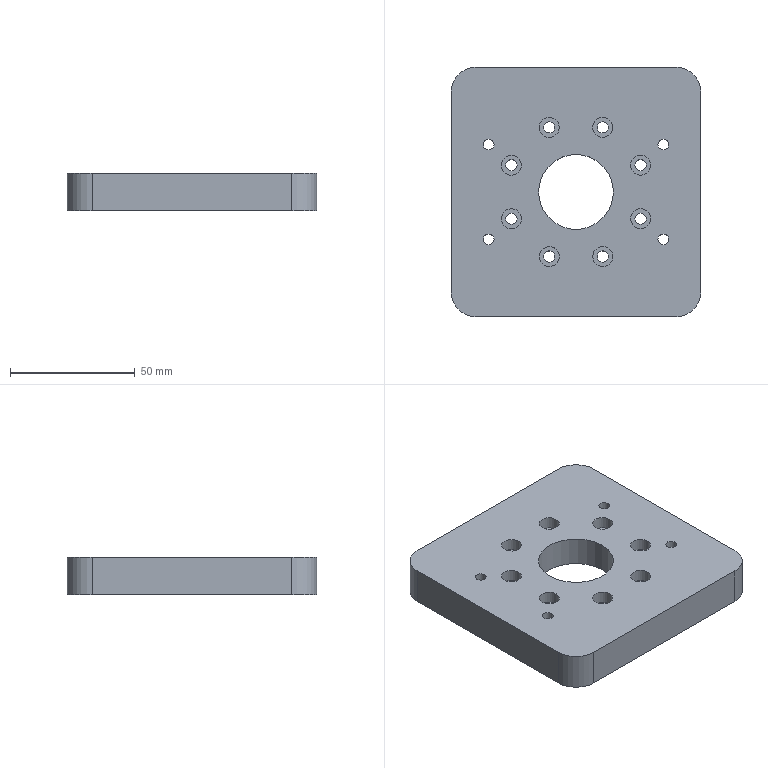NC program | NX | posted with a generic post | part box 100 x 100 x 15 mm
Lines 1 to 24 of 2115:
N10 G17 G21 G94 G90
(FLOOR_WALL_1 , TOOL : D63)
N12 T01 M6
N14 G54
N16 G17 G0 G90 X-86.5 Y51.997 S6500 M3
N18 G43 Z30. H1
N20 Z3.
N22 G94 G1 Z0. F1500.
N24 X-83.5
N26 X83.5
N28 Y25.731
N30 X-83.5
N32 Y-0.534
N34 X83.5
N36 Y-26.8
N38 X-83.5
N40 X-86.5
N42 Z3.
N44 G0 Z30.
N46 M5